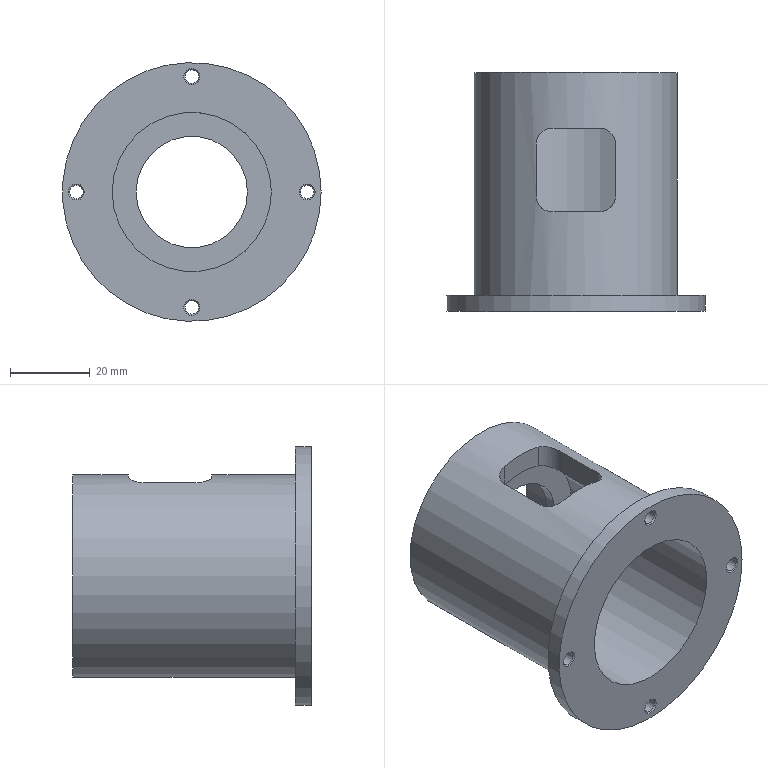Part | NX | features DATUM_CSYS 7, SKETCH 6, EXTRUDE 5, SIMPLE HOLE 4, BLEND 1, HOLE PACKAGE 1 | 1 solid | 30 faces | box 65 x 60 x 65 mm | volume 55807 mm3 | cylinder 13 | plane 9 | cone 8 | commonest cylinder face diameters 3.4 x4 8 x4 28 x1 32 x1 40 x1 51 x1
STEP:
#1=CARTESIAN_POINT('',(20.,48.,0.));
#2=VERTEX_POINT('',#1);
#3=CARTESIAN_POINT('',(0.,48.,0.));
#4=DIRECTION('',(0.,1.,0.));
#5=DIRECTION('',(1.,0.,0.));
#6=AXIS2_PLACEMENT_3D('',#3,#4,#5);
#7=CIRCLE('',#6,20.);
#8=EDGE_CURVE('',#2,#2,#7,.T.);
#9=ORIENTED_EDGE('',*,*,#8,.T.);
#10=EDGE_LOOP('',(#9));
#11=FACE_BOUND('',#10,.T.);
#12=CARTESIAN_POINT('',(20.,0.,0.));
#13=VERTEX_POINT('',#12);
#14=CARTESIAN_POINT('',(0.,0.,0.));
#15=DIRECTION('',(0.,-1.,0.));
#16=DIRECTION('',(1.,0.,0.));
#17=AXIS2_PLACEMENT_3D('',#14,#15,#16);
#18=CIRCLE('',#17,20.);
#19=EDGE_CURVE('',#13,#13,#18,.T.);
#20=ORIENTED_EDGE('',*,*,#19,.T.);
#21=EDGE_LOOP('',(#20));
#22=FACE_BOUND('',#21,.T.);
#23=CARTESIAN_POINT('',(-10.,29.,17.321));
#24=VERTEX_POINT('',#23);
#25=CARTESIAN_POINT('',(-10.,42.,17.321));
#26=VERTEX_POINT('',#25);
#27=CARTESIAN_POINT('',(-10.,4.,17.321));
#28=DIRECTION('',(0.,-1.,0.));
#29=VECTOR('',#28,1000.);
#30=LINE('',#27,#29);
#31=EDGE_CURVE('',#24,#26,#30,.F.);
#32=ORIENTED_EDGE('',*,*,#31,.F.);
#33=CARTESIAN_POINT('',(-6.,25.,19.079));
#34=VERTEX_POINT('',#33);
#35=CARTESIAN_POINT('',(-10.,29.,17.321));
#36=CARTESIAN_POINT('',(-10.,27.896,17.321));
#37=CARTESIAN_POINT('',(-9.05,25.815,17.898));
#38=CARTESIAN_POINT('',(-7.051,25.,18.748));
#39=CARTESIAN_POINT('',(-6.,25.,19.079));
#40=B_SPLINE_CURVE_WITH_KNOTS('',3,(#35,#36,#37,#38,#39),.UNSPECIFIED.,.F.,.F.,(4,1,4),(0.,0.003261,0.006523),.UNSPECIFIED.);
#41=EDGE_CURVE('',#24,#34,#40,.T.);
#42=ORIENTED_EDGE('',*,*,#41,.T.);
#43=CARTESIAN_POINT('',(6.,25.,19.079));
#44=VERTEX_POINT('',#43);
#45=CARTESIAN_POINT('',(0.,25.,0.));
#46=DIRECTION('',(0.,1.,0.));
#47=DIRECTION('',(0.,0.,1.));
#48=AXIS2_PLACEMENT_3D('',#45,#46,#47);
#49=CIRCLE('',#48,20.);
#50=EDGE_CURVE('',#44,#34,#49,.F.);
#51=ORIENTED_EDGE('',*,*,#50,.F.);
#52=CARTESIAN_POINT('',(10.,29.,17.321));
#53=VERTEX_POINT('',#52);
#54=CARTESIAN_POINT('',(6.,25.,19.079));
#55=CARTESIAN_POINT('',(7.053,25.,18.748));
#56=CARTESIAN_POINT('',(9.049,25.816,17.898));
#57=CARTESIAN_POINT('',(10.,27.894,17.321));
#58=CARTESIAN_POINT('',(10.,29.,17.321));
#59=B_SPLINE_CURVE_WITH_KNOTS('',3,(#54,#55,#56,#57,#58),.UNSPECIFIED.,.F.,.F.,(4,1,4),(0.,0.003262,0.006524),.UNSPECIFIED.);
#60=EDGE_CURVE('',#44,#53,#59,.T.);
#61=ORIENTED_EDGE('',*,*,#60,.T.);
#62=CARTESIAN_POINT('',(10.,42.,17.321));
#63=VERTEX_POINT('',#62);
#64=CARTESIAN_POINT('',(10.,4.,17.321));
#65=DIRECTION('',(0.,-1.,0.));
#66=VECTOR('',#65,1000.);
#67=LINE('',#64,#66);
#68=EDGE_CURVE('',#63,#53,#67,.T.);
#69=ORIENTED_EDGE('',*,*,#68,.F.);
#70=CARTESIAN_POINT('',(6.,46.,19.079));
#71=VERTEX_POINT('',#70);
#72=CARTESIAN_POINT('',(10.,42.,17.321));
#73=CARTESIAN_POINT('',(10.,43.104,17.321));
#74=CARTESIAN_POINT('',(9.05,45.185,17.898));
#75=CARTESIAN_POINT('',(7.051,46.,18.748));
#76=CARTESIAN_POINT('',(6.,46.,19.079));
#77=B_SPLINE_CURVE_WITH_KNOTS('',3,(#72,#73,#74,#75,#76),.UNSPECIFIED.,.F.,.F.,(4,1,4),(0.,0.003261,0.006523),.UNSPECIFIED.);
#78=EDGE_CURVE('',#63,#71,#77,.T.);
#79=ORIENTED_EDGE('',*,*,#78,.T.);
#80=CARTESIAN_POINT('',(-6.,46.,19.079));
#81=VERTEX_POINT('',#80);
#82=CARTESIAN_POINT('',(0.,46.,0.));
#83=DIRECTION('',(0.,-1.,0.));
#84=DIRECTION('',(0.,0.,-1.));
#85=AXIS2_PLACEMENT_3D('',#82,#83,#84);
#86=CIRCLE('',#85,20.);
#87=EDGE_CURVE('',#81,#71,#86,.F.);
#88=ORIENTED_EDGE('',*,*,#87,.F.);
#89=CARTESIAN_POINT('',(-6.,46.,19.079));
#90=CARTESIAN_POINT('',(-7.053,46.,18.748));
#91=CARTESIAN_POINT('',(-9.049,45.184,17.898));
#92=CARTESIAN_POINT('',(-10.,43.106,17.321));
#93=CARTESIAN_POINT('',(-10.,42.,17.321));
#94=B_SPLINE_CURVE_WITH_KNOTS('',3,(#89,#90,#91,#92,#93),.UNSPECIFIED.,.F.,.F.,(4,1,4),(0.,0.003262,0.006524),.UNSPECIFIED.);
#95=EDGE_CURVE('',#81,#26,#94,.T.);
#96=ORIENTED_EDGE('',*,*,#95,.T.);
#97=EDGE_LOOP('',(#32,#42,#51,#61,#69,#79,#88,#96));
#98=FACE_BOUND('',#97,.T.);
#99=CARTESIAN_POINT('',(0.,4.,0.));
#100=DIRECTION('',(0.,-1.,0.));
#101=DIRECTION('',(0.,0.,-1.));
#102=AXIS2_PLACEMENT_3D('',#99,#100,#101);
#103=CYLINDRICAL_SURFACE('',#102,20.);
#104=ADVANCED_FACE('',(#11,#22,#98),#103,.F.);
#105=CARTESIAN_POINT('',(25.5,60.,0.));
#106=VERTEX_POINT('',#105);
#107=CARTESIAN_POINT('',(0.,60.,0.));
#108=DIRECTION('',(0.,1.,0.));
#109=DIRECTION('',(1.,0.,0.));
#110=AXIS2_PLACEMENT_3D('',#107,#108,#109);
#111=CIRCLE('',#110,25.5);
#112=EDGE_CURVE('',#106,#106,#111,.T.);
#113=ORIENTED_EDGE('',*,*,#112,.F.);
#114=EDGE_LOOP('',(#113));
#115=FACE_BOUND('',#114,.T.);
#116=CARTESIAN_POINT('',(25.5,4.,0.));
#117=VERTEX_POINT('',#116);
#118=CARTESIAN_POINT('',(0.,4.,0.));
#119=DIRECTION('',(0.,1.,0.));
#120=DIRECTION('',(1.,0.,0.));
#121=AXIS2_PLACEMENT_3D('',#118,#119,#120);
#122=CIRCLE('',#121,25.5);
#123=EDGE_CURVE('',#117,#117,#122,.T.);
#124=ORIENTED_EDGE('',*,*,#123,.T.);
#125=EDGE_LOOP('',(#124));
#126=FACE_BOUND('',#125,.T.);
#127=CARTESIAN_POINT('',(-10.,42.,23.457));
#128=VERTEX_POINT('',#127);
#129=CARTESIAN_POINT('',(-10.,29.,23.457));
#130=VERTEX_POINT('',#129);
#131=CARTESIAN_POINT('',(-10.,48.,23.457));
#132=DIRECTION('',(0.,-1.,0.));
#133=VECTOR('',#132,1000.);
#134=LINE('',#131,#133);
#135=EDGE_CURVE('',#128,#130,#134,.T.);
#136=ORIENTED_EDGE('',*,*,#135,.F.);
#137=CARTESIAN_POINT('',(-6.,46.,24.784));
#138=VERTEX_POINT('',#137);
#139=CARTESIAN_POINT('',(-10.,42.,23.457));
#140=CARTESIAN_POINT('',(-10.,43.084,23.457));
#141=CARTESIAN_POINT('',(-9.082,45.163,23.871));
#142=CARTESIAN_POINT('',(-7.052,46.,24.529));
#143=CARTESIAN_POINT('',(-6.,46.,24.784));
#144=B_SPLINE_CURVE_WITH_KNOTS('',3,(#139,#140,#141,#142,#143),.UNSPECIFIED.,.F.,.F.,(4,1,4),(0.,0.003204,0.006407),.UNSPECIFIED.);
#145=EDGE_CURVE('',#128,#138,#144,.T.);
#146=ORIENTED_EDGE('',*,*,#145,.T.);
#147=CARTESIAN_POINT('',(6.,46.,24.784));
#148=VERTEX_POINT('',#147);
#149=CARTESIAN_POINT('',(0.,46.,0.));
#150=DIRECTION('',(0.,-1.,0.));
#151=DIRECTION('',(0.,0.,-1.));
#152=AXIS2_PLACEMENT_3D('',#149,#150,#151);
#153=CIRCLE('',#152,25.5);
#154=EDGE_CURVE('',#148,#138,#153,.T.);
#155=ORIENTED_EDGE('',*,*,#154,.F.);
#156=CARTESIAN_POINT('',(10.,42.,23.457));
#157=VERTEX_POINT('',#156);
#158=CARTESIAN_POINT('',(6.,46.,24.784));
#159=CARTESIAN_POINT('',(7.053,46.,24.529));
#160=CARTESIAN_POINT('',(9.079,45.165,23.871));
#161=CARTESIAN_POINT('',(10.,43.085,23.457));
#162=CARTESIAN_POINT('',(10.,42.,23.457));
#163=B_SPLINE_CURVE_WITH_KNOTS('',3,(#158,#159,#160,#161,#162),.UNSPECIFIED.,.F.,.F.,(4,1,4),(0.,0.003204,0.006407),.UNSPECIFIED.);
#164=EDGE_CURVE('',#148,#157,#163,.T.);
#165=ORIENTED_EDGE('',*,*,#164,.T.);
#166=CARTESIAN_POINT('',(10.,29.,23.457));
#167=VERTEX_POINT('',#166);
#168=CARTESIAN_POINT('',(10.,48.,23.457));
#169=DIRECTION('',(0.,-1.,0.));
#170=VECTOR('',#169,1000.);
#171=LINE('',#168,#170);
#172=EDGE_CURVE('',#167,#157,#171,.F.);
#173=ORIENTED_EDGE('',*,*,#172,.F.);
#174=CARTESIAN_POINT('',(6.,25.,24.784));
#175=VERTEX_POINT('',#174);
#176=CARTESIAN_POINT('',(10.,29.,23.457));
#177=CARTESIAN_POINT('',(10.,27.916,23.457));
#178=CARTESIAN_POINT('',(9.082,25.837,23.871));
#179=CARTESIAN_POINT('',(7.052,25.,24.529));
#180=CARTESIAN_POINT('',(6.,25.,24.784));
#181=B_SPLINE_CURVE_WITH_KNOTS('',3,(#176,#177,#178,#179,#180),.UNSPECIFIED.,.F.,.F.,(4,1,4),(0.,0.003204,0.006407),.UNSPECIFIED.);
#182=EDGE_CURVE('',#167,#175,#181,.T.);
#183=ORIENTED_EDGE('',*,*,#182,.T.);
#184=CARTESIAN_POINT('',(-6.,25.,24.784));
#185=VERTEX_POINT('',#184);
#186=CARTESIAN_POINT('',(0.,25.,0.));
#187=DIRECTION('',(0.,1.,0.));
#188=DIRECTION('',(0.,0.,1.));
#189=AXIS2_PLACEMENT_3D('',#186,#187,#188);
#190=CIRCLE('',#189,25.5);
#191=EDGE_CURVE('',#185,#175,#190,.T.);
#192=ORIENTED_EDGE('',*,*,#191,.F.);
#193=CARTESIAN_POINT('',(-6.,25.,24.784));
#194=CARTESIAN_POINT('',(-7.053,25.,24.529));
#195=CARTESIAN_POINT('',(-9.079,25.835,23.871));
#196=CARTESIAN_POINT('',(-10.,27.915,23.457));
#197=CARTESIAN_POINT('',(-10.,29.,23.457));
#198=B_SPLINE_CURVE_WITH_KNOTS('',3,(#193,#194,#195,#196,#197),.UNSPECIFIED.,.F.,.F.,(4,1,4),(0.,0.003204,0.006407),.UNSPECIFIED.);
#199=EDGE_CURVE('',#185,#130,#198,.T.);
#200=ORIENTED_EDGE('',*,*,#199,.T.);
#201=EDGE_LOOP('',(#136,#146,#155,#165,#173,#183,#192,#200));
#202=FACE_BOUND('',#201,.T.);
#203=CARTESIAN_POINT('',(0.,48.,0.));
#204=DIRECTION('',(0.,-1.,0.));
#205=DIRECTION('',(0.,0.,-1.));
#206=AXIS2_PLACEMENT_3D('',#203,#204,#205);
#207=CYLINDRICAL_SURFACE('',#206,25.5);
#208=ADVANCED_FACE('',(#115,#126,#202),#207,.T.);
#209=CARTESIAN_POINT('',(14.,51.,0.));
#210=VERTEX_POINT('',#209);
#211=CARTESIAN_POINT('',(0.,51.,0.));
#212=DIRECTION('',(0.,1.,0.));
#213=DIRECTION('',(1.,0.,0.));
#214=AXIS2_PLACEMENT_3D('',#211,#212,#213);
#215=CIRCLE('',#214,14.);
#216=EDGE_CURVE('',#210,#210,#215,.T.);
#217=ORIENTED_EDGE('',*,*,#216,.F.);
#218=EDGE_LOOP('',(#217));
#219=FACE_BOUND('',#218,.T.);
#220=CARTESIAN_POINT('',(16.,51.,0.));
#221=VERTEX_POINT('',#220);
#222=CARTESIAN_POINT('',(0.,51.,0.));
#223=DIRECTION('',(0.,1.,0.));
#224=DIRECTION('',(1.,0.,0.));
#225=AXIS2_PLACEMENT_3D('',#222,#223,#224);
#226=CIRCLE('',#225,16.);
#227=EDGE_CURVE('',#221,#221,#226,.T.);
#228=ORIENTED_EDGE('',*,*,#227,.T.);
#229=EDGE_LOOP('',(#228));
#230=FACE_BOUND('',#229,.T.);
#231=CARTESIAN_POINT('',(0.,51.,0.));
#232=DIRECTION('',(0.,1.,0.));
#233=DIRECTION('',(0.,0.,1.));
#234=AXIS2_PLACEMENT_3D('',#231,#232,#233);
#235=PLANE('',#234);
#236=ADVANCED_FACE('',(#219,#230),#235,.T.);
#237=CARTESIAN_POINT('',(29.,4.,-2.));
#238=VERTEX_POINT('',#237);
#239=CARTESIAN_POINT('',(29.,4.,0.));
#240=DIRECTION('',(0.,-1.,0.));
#241=DIRECTION('',(0.,0.,-1.));
#242=AXIS2_PLACEMENT_3D('',#239,#240,#241);
#243=CIRCLE('',#242,2.);
#244=EDGE_CURVE('',#238,#238,#243,.T.);
#245=ORIENTED_EDGE('',*,*,#244,.T.);
#246=EDGE_LOOP('',(#245));
#247=FACE_BOUND('',#246,.T.);
#248=CARTESIAN_POINT('',(0.,4.,27.));
#249=VERTEX_POINT('',#248);
#250=CARTESIAN_POINT('',(0.,4.,29.));
#251=DIRECTION('',(0.,-1.,0.));
#252=DIRECTION('',(0.,0.,-1.));
#253=AXIS2_PLACEMENT_3D('',#250,#251,#252);
#254=CIRCLE('',#253,2.);
#255=EDGE_CURVE('',#249,#249,#254,.T.);
#256=ORIENTED_EDGE('',*,*,#255,.T.);
#257=EDGE_LOOP('',(#256));
#258=FACE_BOUND('',#257,.T.);
#259=CARTESIAN_POINT('',(0.,4.,-31.));
#260=VERTEX_POINT('',#259);
#261=CARTESIAN_POINT('',(0.,4.,-29.));
#262=DIRECTION('',(0.,-1.,0.));
#263=DIRECTION('',(0.,0.,-1.));
#264=AXIS2_PLACEMENT_3D('',#261,#262,#263);
#265=CIRCLE('',#264,2.);
#266=EDGE_CURVE('',#260,#260,#265,.T.);
#267=ORIENTED_EDGE('',*,*,#266,.T.);
#268=EDGE_LOOP('',(#267));
#269=FACE_BOUND('',#268,.T.);
#270=CARTESIAN_POINT('',(-29.,4.,-2.));
#271=VERTEX_POINT('',#270);
#272=CARTESIAN_POINT('',(-29.,4.,0.));
#273=DIRECTION('',(0.,-1.,0.));
#274=DIRECTION('',(0.,0.,-1.));
#275=AXIS2_PLACEMENT_3D('',#272,#273,#274);
#276=CIRCLE('',#275,2.);
#277=EDGE_CURVE('',#271,#271,#276,.T.);
#278=ORIENTED_EDGE('',*,*,#277,.T.);
#279=EDGE_LOOP('',(#278));
#280=FACE_BOUND('',#279,.T.);
#281=CARTESIAN_POINT('',(32.5,4.,0.));
#282=VERTEX_POINT('',#281);
#283=CARTESIAN_POINT('',(0.,4.,0.));
#284=DIRECTION('',(0.,-1.,0.));
#285=DIRECTION('',(1.,0.,0.));
#286=AXIS2_PLACEMENT_3D('',#283,#284,#285);
#287=CIRCLE('',#286,32.5);
#288=EDGE_CURVE('',#282,#282,#287,.T.);
#289=ORIENTED_EDGE('',*,*,#288,.F.);
#290=EDGE_LOOP('',(#289));
#291=FACE_BOUND('',#290,.T.);
#292=ORIENTED_EDGE('',*,*,#123,.F.);
#293=EDGE_LOOP('',(#292));
#294=FACE_BOUND('',#293,.T.);
#295=CARTESIAN_POINT('',(0.,4.,0.));
#296=DIRECTION('',(0.,-1.,0.));
#297=DIRECTION('',(0.,0.,-1.));
#298=AXIS2_PLACEMENT_3D('',#295,#296,#297);
#299=PLANE('',#298);
#300=ADVANCED_FACE('',(#247,#258,#269,#280,#291,#294),#299,.F.);
#301=ORIENTED_EDGE('',*,*,#288,.T.);
#302=EDGE_LOOP('',(#301));
#303=FACE_BOUND('',#302,.T.);
#304=CARTESIAN_POINT('',(32.5,0.,0.));
#305=VERTEX_POINT('',#304);
#306=CARTESIAN_POINT('',(0.,0.,0.));
#307=DIRECTION('',(0.,-1.,0.));
#308=DIRECTION('',(1.,0.,0.));
#309=AXIS2_PLACEMENT_3D('',#306,#307,#308);
#310=CIRCLE('',#309,32.5);
#311=EDGE_CURVE('',#305,#305,#310,.T.);
#312=ORIENTED_EDGE('',*,*,#311,.F.);
#313=EDGE_LOOP('',(#312));
#314=FACE_BOUND('',#313,.T.);
#315=CARTESIAN_POINT('',(0.,4.,0.));
#316=DIRECTION('',(0.,-1.,0.));
#317=DIRECTION('',(0.,0.,-1.));
#318=AXIS2_PLACEMENT_3D('',#315,#316,#317);
#319=CYLINDRICAL_SURFACE('',#318,32.5);
#320=ADVANCED_FACE('',(#303,#314),#319,.T.);
#321=CARTESIAN_POINT('',(29.,0.,-2.));
#322=VERTEX_POINT('',#321);
#323=CARTESIAN_POINT('',(29.,0.,0.));
#324=DIRECTION('',(0.,-1.,0.));
#325=DIRECTION('',(0.,0.,-1.));
#326=AXIS2_PLACEMENT_3D('',#323,#324,#325);
#327=CIRCLE('',#326,2.);
#328=EDGE_CURVE('',#322,#322,#327,.F.);
#329=ORIENTED_EDGE('',*,*,#328,.T.);
#330=EDGE_LOOP('',(#329));
#331=FACE_BOUND('',#330,.T.);
#332=CARTESIAN_POINT('',(0.,0.,27.));
#333=VERTEX_POINT('',#332);
#334=CARTESIAN_POINT('',(0.,0.,29.));
#335=DIRECTION('',(0.,-1.,0.));
#336=DIRECTION('',(0.,0.,-1.));
#337=AXIS2_PLACEMENT_3D('',#334,#335,#336);
#338=CIRCLE('',#337,2.);
#339=EDGE_CURVE('',#333,#333,#338,.F.);
#340=ORIENTED_EDGE('',*,*,#339,.T.);
#341=EDGE_LOOP('',(#340));
#342=FACE_BOUND('',#341,.T.);
#343=CARTESIAN_POINT('',(0.,0.,-31.));
#344=VERTEX_POINT('',#343);
#345=CARTESIAN_POINT('',(0.,0.,-29.));
#346=DIRECTION('',(0.,-1.,0.));
#347=DIRECTION('',(0.,0.,-1.));
#348=AXIS2_PLACEMENT_3D('',#345,#346,#347);
#349=CIRCLE('',#348,2.);
#350=EDGE_CURVE('',#344,#344,#349,.F.);
#351=ORIENTED_EDGE('',*,*,#350,.T.);
#352=EDGE_LOOP('',(#351));
#353=FACE_BOUND('',#352,.T.);
#354=CARTESIAN_POINT('',(-29.,0.,-2.));
#355=VERTEX_POINT('',#354);
#356=CARTESIAN_POINT('',(-29.,0.,0.));
#357=DIRECTION('',(0.,-1.,0.));
#358=DIRECTION('',(0.,0.,-1.));
#359=AXIS2_PLACEMENT_3D('',#356,#357,#358);
#360=CIRCLE('',#359,2.);
#361=EDGE_CURVE('',#355,#355,#360,.F.);
#362=ORIENTED_EDGE('',*,*,#361,.T.);
#363=EDGE_LOOP('',(#362));
#364=FACE_BOUND('',#363,.T.);
#365=ORIENTED_EDGE('',*,*,#311,.T.);
#366=EDGE_LOOP('',(#365));
#367=FACE_BOUND('',#366,.T.);
#368=ORIENTED_EDGE('',*,*,#19,.F.);
#369=EDGE_LOOP('',(#368));
#370=FACE_BOUND('',#369,.T.);
#371=CARTESIAN_POINT('',(0.,0.,0.));
#372=DIRECTION('',(0.,-1.,0.));
#373=DIRECTION('',(0.,0.,-1.));
#374=AXIS2_PLACEMENT_3D('',#371,#372,#373);
#375=PLANE('',#374);
#376=ADVANCED_FACE('',(#331,#342,#353,#364,#367,#370),#375,.T.);
#377=ORIENTED_EDGE('',*,*,#216,.T.);
#378=EDGE_LOOP('',(#377));
#379=FACE_BOUND('',#378,.T.);
#380=CARTESIAN_POINT('',(14.,48.,0.));
#381=VERTEX_POINT('',#380);
#382=CARTESIAN_POINT('',(0.,48.,0.));
#383=DIRECTION('',(0.,1.,0.));
#384=DIRECTION('',(1.,0.,0.));
#385=AXIS2_PLACEMENT_3D('',#382,#383,#384);
#386=CIRCLE('',#385,14.);
#387=EDGE_CURVE('',#381,#381,#386,.T.);
#388=ORIENTED_EDGE('',*,*,#387,.F.);
#389=EDGE_LOOP('',(#388));
#390=FACE_BOUND('',#389,.T.);
#391=CARTESIAN_POINT('',(0.,51.,0.));
#392=DIRECTION('',(0.,-1.,0.));
#393=DIRECTION('',(0.,0.,-1.));
#394=AXIS2_PLACEMENT_3D('',#391,#392,#393);
#395=CYLINDRICAL_SURFACE('',#394,14.);
#396=ADVANCED_FACE('',(#379,#390),#395,.F.);
#397=ORIENTED_EDGE('',*,*,#8,.F.);
#398=EDGE_LOOP('',(#397));
#399=FACE_BOUND('',#398,.T.);
#400=ORIENTED_EDGE('',*,*,#387,.T.);
#401=EDGE_LOOP('',(#400));
#402=FACE_BOUND('',#401,.T.);
#403=CARTESIAN_POINT('',(0.,48.,0.));
#404=DIRECTION('',(0.,1.,0.));
#405=DIRECTION('',(0.,0.,1.));
#406=AXIS2_PLACEMENT_3D('',#403,#404,#405);
#407=PLANE('',#406);
#408=ADVANCED_FACE('',(#399,#402),#407,.F.);
#409=CARTESIAN_POINT('',(-29.,3.7,-1.7));
#410=VERTEX_POINT('',#409);
#411=CARTESIAN_POINT('',(-29.,3.7,0.));
#412=DIRECTION('',(0.,-1.,0.));
#413=DIRECTION('',(0.,0.,-1.));
#414=AXIS2_PLACEMENT_3D('',#411,#412,#413);
#415=CIRCLE('',#414,1.7);
#416=EDGE_CURVE('',#410,#410,#415,.F.);
#417=ORIENTED_EDGE('',*,*,#416,.T.);
#418=EDGE_LOOP('',(#417));
#419=FACE_BOUND('',#418,.T.);
#420=CARTESIAN_POINT('',(-29.,0.3,-1.7));
#421=VERTEX_POINT('',#420);
#422=CARTESIAN_POINT('',(-29.,0.3,0.));
#423=DIRECTION('',(0.,-1.,0.));
#424=DIRECTION('',(0.,0.,-1.));
#425=AXIS2_PLACEMENT_3D('',#422,#423,#424);
#426=CIRCLE('',#425,1.7);
#427=EDGE_CURVE('',#421,#421,#426,.T.);
#428=ORIENTED_EDGE('',*,*,#427,.T.);
#429=EDGE_LOOP('',(#428));
#430=FACE_BOUND('',#429,.T.);
#431=CARTESIAN_POINT('',(-29.,0.,0.));
#432=DIRECTION('',(0.,1.,0.));
#433=DIRECTION('',(0.,0.,1.));
#434=AXIS2_PLACEMENT_3D('',#431,#432,#433);
#435=CYLINDRICAL_SURFACE('',#434,1.7);
#436=ADVANCED_FACE('',(#419,#430),#435,.F.);
#437=ORIENTED_EDGE('',*,*,#427,.F.);
#438=EDGE_LOOP('',(#437));
#439=FACE_BOUND('',#438,.T.);
#440=ORIENTED_EDGE('',*,*,#361,.F.);
#441=EDGE_LOOP('',(#440));
#442=FACE_BOUND('',#441,.T.);
#443=CARTESIAN_POINT('',(-29.,0.,0.));
#444=DIRECTION('',(0.,-1.,0.));
#445=DIRECTION('',(0.,0.,-1.));
#446=AXIS2_PLACEMENT_3D('',#443,#444,#445);
#447=CONICAL_SURFACE('',#446,2.,0.7854);
#448=ADVANCED_FACE('',(#439,#442),#447,.F.);
#449=ORIENTED_EDGE('',*,*,#416,.F.);
#450=EDGE_LOOP('',(#449));
#451=FACE_BOUND('',#450,.T.);
#452=ORIENTED_EDGE('',*,*,#277,.F.);
#453=EDGE_LOOP('',(#452));
#454=FACE_BOUND('',#453,.T.);
#455=CARTESIAN_POINT('',(-29.,4.,0.));
#456=DIRECTION('',(0.,1.,0.));
#457=DIRECTION('',(0.,0.,1.));
#458=AXIS2_PLACEMENT_3D('',#455,#456,#457);
#459=CONICAL_SURFACE('',#458,2.,0.7854);
#460=ADVANCED_FACE('',(#451,#454),#459,.F.);
#461=CARTESIAN_POINT('',(0.,3.7,-30.7));
#462=VERTEX_POINT('',#461);
#463=CARTESIAN_POINT('',(0.,3.7,-29.));
#464=DIRECTION('',(0.,-1.,0.));
#465=DIRECTION('',(0.,0.,-1.));
#466=AXIS2_PLACEMENT_3D('',#463,#464,#465);
#467=CIRCLE('',#466,1.7);
#468=EDGE_CURVE('',#462,#462,#467,.F.);
#469=ORIENTED_EDGE('',*,*,#468,.T.);
#470=EDGE_LOOP('',(#469));
#471=FACE_BOUND('',#470,.T.);
#472=CARTESIAN_POINT('',(0.,0.3,-30.7));
#473=VERTEX_POINT('',#472);
#474=CARTESIAN_POINT('',(0.,0.3,-29.));
#475=DIRECTION('',(0.,-1.,0.));
#476=DIRECTION('',(0.,0.,-1.));
#477=AXIS2_PLACEMENT_3D('',#474,#475,#476);
#478=CIRCLE('',#477,1.7);
#479=EDGE_CURVE('',#473,#473,#478,.T.);
#480=ORIENTED_EDGE('',*,*,#479,.T.);
#481=EDGE_LOOP('',(#480));
#482=FACE_BOUND('',#481,.T.);
#483=CARTESIAN_POINT('',(0.,0.,-29.));
#484=DIRECTION('',(0.,1.,0.));
#485=DIRECTION('',(0.,0.,1.));
#486=AXIS2_PLACEMENT_3D('',#483,#484,#485);
#487=CYLINDRICAL_SURFACE('',#486,1.7);
#488=ADVANCED_FACE('',(#471,#482),#487,.F.);
#489=ORIENTED_EDGE('',*,*,#479,.F.);
#490=EDGE_LOOP('',(#489));
#491=FACE_BOUND('',#490,.T.);
#492=ORIENTED_EDGE('',*,*,#350,.F.);
#493=EDGE_LOOP('',(#492));
#494=FACE_BOUND('',#493,.T.);
#495=CARTESIAN_POINT('',(0.,0.,-29.));
#496=DIRECTION('',(0.,-1.,0.));
#497=DIRECTION('',(0.,0.,-1.));
#498=AXIS2_PLACEMENT_3D('',#495,#496,#497);
#499=CONICAL_SURFACE('',#498,2.,0.7854);
#500=ADVANCED_FACE('',(#491,#494),#499,.F.);
#501=ORIENTED_EDGE('',*,*,#468,.F.);
#502=EDGE_LOOP('',(#501));
#503=FACE_BOUND('',#502,.T.);
#504=ORIENTED_EDGE('',*,*,#266,.F.);
#505=EDGE_LOOP('',(#504));
#506=FACE_BOUND('',#505,.T.);
#507=CARTESIAN_POINT('',(0.,4.,-29.));
#508=DIRECTION('',(0.,1.,0.));
#509=DIRECTION('',(0.,0.,1.));
#510=AXIS2_PLACEMENT_3D('',#507,#508,#509);
#511=CONICAL_SURFACE('',#510,2.,0.7854);
#512=ADVANCED_FACE('',(#503,#506),#511,.F.);
#513=CARTESIAN_POINT('',(0.,3.7,27.3));
#514=VERTEX_POINT('',#513);
#515=CARTESIAN_POINT('',(0.,3.7,29.));
#516=DIRECTION('',(0.,-1.,0.));
#517=DIRECTION('',(0.,0.,-1.));
#518=AXIS2_PLACEMENT_3D('',#515,#516,#517);
#519=CIRCLE('',#518,1.7);
#520=EDGE_CURVE('',#514,#514,#519,.F.);
#521=ORIENTED_EDGE('',*,*,#520,.T.);
#522=EDGE_LOOP('',(#521));
#523=FACE_BOUND('',#522,.T.);
#524=CARTESIAN_POINT('',(0.,0.3,27.3));
#525=VERTEX_POINT('',#524);
#526=CARTESIAN_POINT('',(0.,0.3,29.));
#527=DIRECTION('',(0.,-1.,0.));
#528=DIRECTION('',(0.,0.,-1.));
#529=AXIS2_PLACEMENT_3D('',#526,#527,#528);
#530=CIRCLE('',#529,1.7);
#531=EDGE_CURVE('',#525,#525,#530,.T.);
#532=ORIENTED_EDGE('',*,*,#531,.T.);
#533=EDGE_LOOP('',(#532));
#534=FACE_BOUND('',#533,.T.);
#535=CARTESIAN_POINT('',(0.,0.,29.));
#536=DIRECTION('',(0.,1.,0.));
#537=DIRECTION('',(0.,0.,1.));
#538=AXIS2_PLACEMENT_3D('',#535,#536,#537);
#539=CYLINDRICAL_SURFACE('',#538,1.7);
#540=ADVANCED_FACE('',(#523,#534),#539,.F.);
#541=ORIENTED_EDGE('',*,*,#531,.F.);
#542=EDGE_LOOP('',(#541));
#543=FACE_BOUND('',#542,.T.);
#544=ORIENTED_EDGE('',*,*,#339,.F.);
#545=EDGE_LOOP('',(#544));
#546=FACE_BOUND('',#545,.T.);
#547=CARTESIAN_POINT('',(0.,0.,29.));
#548=DIRECTION('',(0.,-1.,0.));
#549=DIRECTION('',(0.,0.,-1.));
#550=AXIS2_PLACEMENT_3D('',#547,#548,#549);
#551=CONICAL_SURFACE('',#550,2.,0.7854);
#552=ADVANCED_FACE('',(#543,#546),#551,.F.);
#553=ORIENTED_EDGE('',*,*,#520,.F.);
#554=EDGE_LOOP('',(#553));
#555=FACE_BOUND('',#554,.T.);
#556=ORIENTED_EDGE('',*,*,#255,.F.);
#557=EDGE_LOOP('',(#556));
#558=FACE_BOUND('',#557,.T.);
#559=CARTESIAN_POINT('',(0.,4.,29.));
#560=DIRECTION('',(0.,1.,0.));
#561=DIRECTION('',(0.,0.,1.));
#562=AXIS2_PLACEMENT_3D('',#559,#560,#561);
#563=CONICAL_SURFACE('',#562,2.,0.7854);
#564=ADVANCED_FACE('',(#555,#558),#563,.F.);
#565=CARTESIAN_POINT('',(29.,3.7,-1.7));
#566=VERTEX_POINT('',#565);
#567=CARTESIAN_POINT('',(29.,3.7,0.));
#568=DIRECTION('',(0.,-1.,0.));
#569=DIRECTION('',(0.,0.,-1.));
#570=AXIS2_PLACEMENT_3D('',#567,#568,#569);
#571=CIRCLE('',#570,1.7);
#572=EDGE_CURVE('',#566,#566,#571,.F.);
#573=ORIENTED_EDGE('',*,*,#572,.T.);
#574=EDGE_LOOP('',(#573));
#575=FACE_BOUND('',#574,.T.);
#576=CARTESIAN_POINT('',(29.,0.3,-1.7));
#577=VERTEX_POINT('',#576);
#578=CARTESIAN_POINT('',(29.,0.3,0.));
#579=DIRECTION('',(0.,-1.,0.));
#580=DIRECTION('',(0.,0.,-1.));
#581=AXIS2_PLACEMENT_3D('',#578,#579,#580);
#582=CIRCLE('',#581,1.7);
#583=EDGE_CURVE('',#577,#577,#582,.T.);
#584=ORIENTED_EDGE('',*,*,#583,.T.);
#585=EDGE_LOOP('',(#584));
#586=FACE_BOUND('',#585,.T.);
#587=CARTESIAN_POINT('',(29.,0.,0.));
#588=DIRECTION('',(0.,1.,0.));
#589=DIRECTION('',(0.,0.,1.));
#590=AXIS2_PLACEMENT_3D('',#587,#588,#589);
#591=CYLINDRICAL_SURFACE('',#590,1.7);
#592=ADVANCED_FACE('',(#575,#586),#591,.F.);
#593=ORIENTED_EDGE('',*,*,#583,.F.);
#594=EDGE_LOOP('',(#593));
#595=FACE_BOUND('',#594,.T.);
#596=ORIENTED_EDGE('',*,*,#328,.F.);
#597=EDGE_LOOP('',(#596));
#598=FACE_BOUND('',#597,.T.);
#599=CARTESIAN_POINT('',(29.,0.,0.));
#600=DIRECTION('',(0.,-1.,0.));
#601=DIRECTION('',(0.,0.,-1.));
#602=AXIS2_PLACEMENT_3D('',#599,#600,#601);
#603=CONICAL_SURFACE('',#602,2.,0.7854);
#604=ADVANCED_FACE('',(#595,#598),#603,.F.);
#605=ORIENTED_EDGE('',*,*,#572,.F.);
#606=EDGE_LOOP('',(#605));
#607=FACE_BOUND('',#606,.T.);
#608=ORIENTED_EDGE('',*,*,#244,.F.);
#609=EDGE_LOOP('',(#608));
#610=FACE_BOUND('',#609,.T.);
#611=CARTESIAN_POINT('',(29.,4.,0.));
#612=DIRECTION('',(0.,1.,0.));
#613=DIRECTION('',(0.,0.,1.));
#614=AXIS2_PLACEMENT_3D('',#611,#612,#613);
#615=CONICAL_SURFACE('',#614,2.,0.7854);
#616=ADVANCED_FACE('',(#607,#610),#615,.F.);
#617=CARTESIAN_POINT('',(16.,60.,0.));
#618=VERTEX_POINT('',#617);
#619=CARTESIAN_POINT('',(0.,60.,0.));
#620=DIRECTION('',(0.,1.,0.));
#621=DIRECTION('',(1.,0.,0.));
#622=AXIS2_PLACEMENT_3D('',#619,#620,#621);
#623=CIRCLE('',#622,16.);
#624=EDGE_CURVE('',#618,#618,#623,.T.);
#625=ORIENTED_EDGE('',*,*,#624,.T.);
#626=EDGE_LOOP('',(#625));
#627=FACE_BOUND('',#626,.T.);
#628=ORIENTED_EDGE('',*,*,#227,.F.);
#629=EDGE_LOOP('',(#628));
#630=FACE_BOUND('',#629,.T.);
#631=CARTESIAN_POINT('',(0.,60.,0.));
#632=DIRECTION('',(0.,-1.,0.));
#633=DIRECTION('',(0.,0.,-1.));
#634=AXIS2_PLACEMENT_3D('',#631,#632,#633);
#635=CYLINDRICAL_SURFACE('',#634,16.);
#636=ADVANCED_FACE('',(#627,#630),#635,.F.);
#637=ORIENTED_EDGE('',*,*,#112,.T.);
#638=EDGE_LOOP('',(#637));
#639=FACE_BOUND('',#638,.T.);
#640=ORIENTED_EDGE('',*,*,#624,.F.);
#641=EDGE_LOOP('',(#640));
#642=FACE_BOUND('',#641,.T.);
#643=CARTESIAN_POINT('',(0.,60.,0.));
#644=DIRECTION('',(0.,1.,0.));
#645=DIRECTION('',(0.,0.,1.));
#646=AXIS2_PLACEMENT_3D('',#643,#644,#645);
#647=PLANE('',#646);
#648=ADVANCED_FACE('',(#639,#642),#647,.T.);
#649=ORIENTED_EDGE('',*,*,#31,.T.);
#650=CARTESIAN_POINT('',(-10.,42.,23.457));
#651=DIRECTION('',(0.,0.,1.));
#652=VECTOR('',#651,1000.);
#653=LINE('',#650,#652);
#654=EDGE_CURVE('',#26,#128,#653,.T.);
#655=ORIENTED_EDGE('',*,*,#654,.T.);
#656=ORIENTED_EDGE('',*,*,#135,.T.);
#657=CARTESIAN_POINT('',(-10.,29.,17.321));
#658=DIRECTION('',(0.,0.,1.));
#659=VECTOR('',#658,1000.);
#660=LINE('',#657,#659);
#661=EDGE_CURVE('',#130,#24,#660,.F.);
#662=ORIENTED_EDGE('',*,*,#661,.T.);
#663=EDGE_LOOP('',(#649,#655,#656,#662));
#664=FACE_BOUND('',#663,.T.);
#665=CARTESIAN_POINT('',(-10.,46.,50.));
#666=DIRECTION('',(1.,0.,0.));
#667=DIRECTION('',(0.,1.,0.));
#668=AXIS2_PLACEMENT_3D('',#665,#666,#667);
#669=PLANE('',#668);
#670=ADVANCED_FACE('',(#664),#669,.T.);
#671=ORIENTED_EDGE('',*,*,#191,.T.);
#672=CARTESIAN_POINT('',(6.,25.,17.321));
#673=DIRECTION('',(0.,0.,1.));
#674=VECTOR('',#673,1000.);
#675=LINE('',#672,#674);
#676=EDGE_CURVE('',#175,#44,#675,.F.);
#677=ORIENTED_EDGE('',*,*,#676,.T.);
#678=ORIENTED_EDGE('',*,*,#50,.T.);
#679=CARTESIAN_POINT('',(-6.,25.,23.457));
#680=DIRECTION('',(0.,0.,1.));
#681=VECTOR('',#680,1000.);
#682=LINE('',#679,#681);
#683=EDGE_CURVE('',#34,#185,#682,.T.);
#684=ORIENTED_EDGE('',*,*,#683,.T.);
#685=EDGE_LOOP('',(#671,#677,#678,#684));
#686=FACE_BOUND('',#685,.T.);
#687=CARTESIAN_POINT('',(-10.,25.,50.));
#688=DIRECTION('',(0.,1.,0.));
#689=DIRECTION('',(0.,0.,1.));
#690=AXIS2_PLACEMENT_3D('',#687,#688,#689);
#691=PLANE('',#690);
#692=ADVANCED_FACE('',(#686),#691,.T.);
#693=ORIENTED_EDGE('',*,*,#172,.T.);
#694=CARTESIAN_POINT('',(10.,42.,17.321));
#695=DIRECTION('',(0.,0.,1.));
#696=VECTOR('',#695,1000.);
#697=LINE('',#694,#696);
#698=EDGE_CURVE('',#157,#63,#697,.F.);
#699=ORIENTED_EDGE('',*,*,#698,.T.);
#700=ORIENTED_EDGE('',*,*,#68,.T.);
#701=CARTESIAN_POINT('',(10.,29.,23.457));
#702=DIRECTION('',(0.,0.,1.));
#703=VECTOR('',#702,1000.);
#704=LINE('',#701,#703);
#705=EDGE_CURVE('',#53,#167,#704,.T.);
#706=ORIENTED_EDGE('',*,*,#705,.T.);
#707=EDGE_LOOP('',(#693,#699,#700,#706));
#708=FACE_BOUND('',#707,.T.);
#709=CARTESIAN_POINT('',(10.,25.,50.));
#710=DIRECTION('',(-1.,0.,0.));
#711=DIRECTION('',(0.,-1.,0.));
#712=AXIS2_PLACEMENT_3D('',#709,#710,#711);
#713=PLANE('',#712);
#714=ADVANCED_FACE('',(#708),#713,.T.);
#715=ORIENTED_EDGE('',*,*,#87,.T.);
#716=CARTESIAN_POINT('',(6.,46.,23.457));
#717=DIRECTION('',(0.,0.,1.));
#718=VECTOR('',#717,1000.);
#719=LINE('',#716,#718);
#720=EDGE_CURVE('',#71,#148,#719,.T.);
#721=ORIENTED_EDGE('',*,*,#720,.T.);
#722=ORIENTED_EDGE('',*,*,#154,.T.);
#723=CARTESIAN_POINT('',(-6.,46.,17.321));
#724=DIRECTION('',(0.,0.,1.));
#725=VECTOR('',#724,1000.);
#726=LINE('',#723,#725);
#727=EDGE_CURVE('',#138,#81,#726,.F.);
#728=ORIENTED_EDGE('',*,*,#727,.T.);
#729=EDGE_LOOP('',(#715,#721,#722,#728));
#730=FACE_BOUND('',#729,.T.);
#731=CARTESIAN_POINT('',(10.,46.,50.));
#732=DIRECTION('',(0.,-1.,0.));
#733=DIRECTION('',(0.,0.,-1.));
#734=AXIS2_PLACEMENT_3D('',#731,#732,#733);
#735=PLANE('',#734);
#736=ADVANCED_FACE('',(#730),#735,.T.);
#737=ORIENTED_EDGE('',*,*,#78,.F.);
#738=ORIENTED_EDGE('',*,*,#698,.F.);
#739=ORIENTED_EDGE('',*,*,#164,.F.);
#740=ORIENTED_EDGE('',*,*,#720,.F.);
#741=EDGE_LOOP('',(#737,#738,#739,#740));
#742=FACE_BOUND('',#741,.T.);
#743=CARTESIAN_POINT('',(6.,42.,50.));
#744=DIRECTION('',(0.,0.,-1.));
#745=DIRECTION('',(-1.,0.,0.));
#746=AXIS2_PLACEMENT_3D('',#743,#744,#745);
#747=CYLINDRICAL_SURFACE('',#746,4.);
#748=ADVANCED_FACE('',(#742),#747,.F.);
#749=ORIENTED_EDGE('',*,*,#60,.F.);
#750=ORIENTED_EDGE('',*,*,#676,.F.);
#751=ORIENTED_EDGE('',*,*,#182,.F.);
#752=ORIENTED_EDGE('',*,*,#705,.F.);
#753=EDGE_LOOP('',(#749,#750,#751,#752));
#754=FACE_BOUND('',#753,.T.);
#755=CARTESIAN_POINT('',(6.,29.,50.));
#756=DIRECTION('',(0.,0.,-1.));
#757=DIRECTION('',(-1.,0.,0.));
#758=AXIS2_PLACEMENT_3D('',#755,#756,#757);
#759=CYLINDRICAL_SURFACE('',#758,4.);
#760=ADVANCED_FACE('',(#754),#759,.F.);
#761=ORIENTED_EDGE('',*,*,#95,.F.);
#762=ORIENTED_EDGE('',*,*,#727,.F.);
#763=ORIENTED_EDGE('',*,*,#145,.F.);
#764=ORIENTED_EDGE('',*,*,#654,.F.);
#765=EDGE_LOOP('',(#761,#762,#763,#764));
#766=FACE_BOUND('',#765,.T.);
#767=CARTESIAN_POINT('',(-6.,42.,50.));
#768=DIRECTION('',(0.,0.,-1.));
#769=DIRECTION('',(-1.,0.,0.));
#770=AXIS2_PLACEMENT_3D('',#767,#768,#769);
#771=CYLINDRICAL_SURFACE('',#770,4.);
#772=ADVANCED_FACE('',(#766),#771,.F.);
#773=ORIENTED_EDGE('',*,*,#41,.F.);
#774=ORIENTED_EDGE('',*,*,#661,.F.);
#775=ORIENTED_EDGE('',*,*,#199,.F.);
#776=ORIENTED_EDGE('',*,*,#683,.F.);
#777=EDGE_LOOP('',(#773,#774,#775,#776));
#778=FACE_BOUND('',#777,.T.);
#779=CARTESIAN_POINT('',(-6.,29.,50.));
#780=DIRECTION('',(0.,0.,-1.));
#781=DIRECTION('',(-1.,0.,0.));
#782=AXIS2_PLACEMENT_3D('',#779,#780,#781);
#783=CYLINDRICAL_SURFACE('',#782,4.);
#784=ADVANCED_FACE('',(#778),#783,.F.);
#785=CLOSED_SHELL('',(#104,#208,#236,#300,#320,#376,#396,#408,#436,#448,#460,#488,#500,#512,#540,#552,#564,#592,#604,#616,#636,#648,#670,#692,#714,#736,#748,#760,#772,#784));
#786=MANIFOLD_SOLID_BREP('',#785);
#787=(LENGTH_UNIT()NAMED_UNIT(*)SI_UNIT(.MILLI.,.METRE.));
#788=UNCERTAINTY_MEASURE_WITH_UNIT(LENGTH_MEASURE(0.0508),#787,'','');
#789=(NAMED_UNIT(*)PLANE_ANGLE_UNIT()SI_UNIT($,.RADIAN.));
#790=(NAMED_UNIT(*)SI_UNIT($,.STERADIAN.)SOLID_ANGLE_UNIT());
#791=(GEOMETRIC_REPRESENTATION_CONTEXT(3)GLOBAL_UNCERTAINTY_ASSIGNED_CONTEXT((#788))GLOBAL_UNIT_ASSIGNED_CONTEXT((#787,#789,#790))REPRESENTATION_CONTEXT('',''));
#792=ADVANCED_BREP_SHAPE_REPRESENTATION('',(#786),#791);